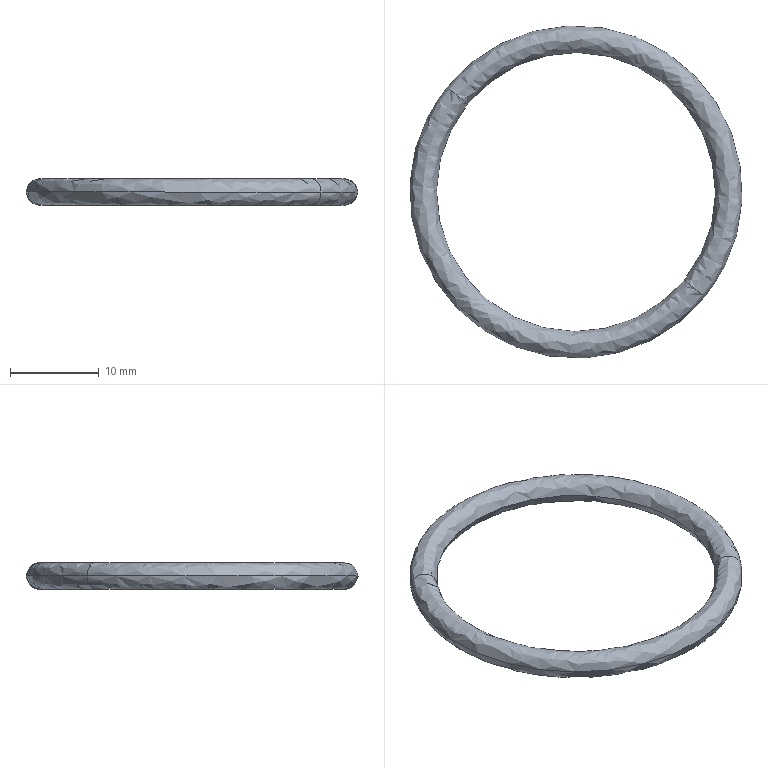Part | SolidWorks | features BaseBody 1 | 1 solid | 4 faces | box 37.4 x 37.4 x 3 mm | volume 763.908 mm3 | spline 4
STEP:
#1=CARTESIAN_POINT('',(521.677,-144.086,275.815));
#2=VERTEX_POINT('',#1);
#3=CARTESIAN_POINT('',(497.316,-124.275,275.815));
#4=VERTEX_POINT('',#3);
#5=CARTESIAN_POINT('',(509.496,-134.18,275.815));
#6=DIRECTION('',(0.000000024,-0.000000004,1.));
#7=DIRECTION('',(-0.7758,0.6309,0.000000021));
#8=AXIS2_PLACEMENT_3D('',#5,#6,#7);
#9=CIRCLE('',#8,15.7);
#10=EDGE_CURVE('',#2,#4,#9,.T.);
#11=ORIENTED_EDGE('',*,*,#10,.F.);
#12=CARTESIAN_POINT('',(524.004,-145.979,275.815));
#13=VERTEX_POINT('',#12);
#14=CARTESIAN_POINT('',(522.841,-145.032,275.815));
#15=DIRECTION('',(0.6309,0.7758,-0.000000012));
#16=DIRECTION('',(0.7758,-0.6309,-0.000000021));
#17=AXIS2_PLACEMENT_3D('',#14,#15,#16);
#18=CIRCLE('',#17,1.5);
#19=EDGE_CURVE('',#2,#13,#18,.T.);
#20=ORIENTED_EDGE('',*,*,#19,.T.);
#21=CARTESIAN_POINT('',(494.988,-122.382,275.815));
#22=VERTEX_POINT('',#21);
#23=CARTESIAN_POINT('',(509.496,-134.18,275.815));
#24=DIRECTION('',(0.000000024,-0.000000004,1.));
#25=DIRECTION('',(-0.7758,0.6309,0.000000021));
#26=AXIS2_PLACEMENT_3D('',#23,#24,#25);
#27=CIRCLE('',#26,18.7);
#28=EDGE_CURVE('',#13,#22,#27,.T.);
#29=ORIENTED_EDGE('',*,*,#28,.T.);
#30=CARTESIAN_POINT('',(496.152,-123.329,275.815));
#31=DIRECTION('',(-0.6309,-0.7758,0.000000012));
#32=DIRECTION('',(-0.7758,0.6309,0.000000021));
#33=AXIS2_PLACEMENT_3D('',#30,#31,#32);
#34=CIRCLE('',#33,1.5);
#35=EDGE_CURVE('',#4,#22,#34,.T.);
#36=ORIENTED_EDGE('',*,*,#35,.F.);
#37=EDGE_LOOP('',(#11,#20,#29,#36));
#38=FACE_OUTER_BOUND('',#37,.T.);
#39=CARTESIAN_POINT('',(521.677,-144.086,275.815));
#40=CARTESIAN_POINT('',(541.488,-119.725,275.815));
#41=CARTESIAN_POINT('',(517.127,-99.914,275.815));
#42=CARTESIAN_POINT('',(497.316,-124.275,275.815));
#43=CARTESIAN_POINT('',(521.677,-144.086,278.815));
#44=CARTESIAN_POINT('',(541.488,-119.725,278.815));
#45=CARTESIAN_POINT('',(517.127,-99.914,278.815));
#46=CARTESIAN_POINT('',(497.316,-124.275,278.815));
#47=CARTESIAN_POINT('',(524.004,-145.979,278.815));
#48=CARTESIAN_POINT('',(547.601,-116.962,278.815));
#49=CARTESIAN_POINT('',(518.585,-93.366,278.815));
#50=CARTESIAN_POINT('',(494.988,-122.382,278.815));
#51=CARTESIAN_POINT('',(524.004,-145.979,275.815));
#52=CARTESIAN_POINT('',(547.601,-116.962,275.815));
#53=CARTESIAN_POINT('',(518.585,-93.366,275.815));
#54=CARTESIAN_POINT('',(494.988,-122.382,275.815));
#55=(BOUNDED_SURFACE()B_SPLINE_SURFACE(3,3,((#39,#40,#41,#42),(#43,#44,#45,#46),(#47,#48,#49,#50),(#51,#52,#53,#54)),.UNSPECIFIED.,.F.,.F.,.F.)B_SPLINE_SURFACE_WITH_KNOTS((4,4),(4,4),(0.,1.),(0.,1.),.UNSPECIFIED.)GEOMETRIC_REPRESENTATION_ITEM()RATIONAL_B_SPLINE_SURFACE(((1.,0.3333,0.3333,1.),(0.3333,0.1111,0.1111,0.3333),(0.3333,0.1111,0.1111,0.3333),(1.,0.3333,0.3333,1.)))REPRESENTATION_ITEM('')SURFACE());
#56=ADVANCED_FACE('',(#38),#55,.T.);
#57=ORIENTED_EDGE('',*,*,#28,.F.);
#58=CARTESIAN_POINT('',(522.841,-145.032,275.815));
#59=DIRECTION('',(0.6309,0.7758,-0.000000012));
#60=DIRECTION('',(0.7758,-0.6309,-0.000000021));
#61=AXIS2_PLACEMENT_3D('',#58,#59,#60);
#62=CIRCLE('',#61,1.5);
#63=EDGE_CURVE('',#13,#2,#62,.T.);
#64=ORIENTED_EDGE('',*,*,#63,.T.);
#65=ORIENTED_EDGE('',*,*,#10,.T.);
#66=CARTESIAN_POINT('',(496.152,-123.329,275.815));
#67=DIRECTION('',(-0.6309,-0.7758,0.000000012));
#68=DIRECTION('',(-0.7758,0.6309,0.000000021));
#69=AXIS2_PLACEMENT_3D('',#66,#67,#68);
#70=CIRCLE('',#69,1.5);
#71=EDGE_CURVE('',#22,#4,#70,.T.);
#72=ORIENTED_EDGE('',*,*,#71,.F.);
#73=EDGE_LOOP('',(#57,#64,#65,#72));
#74=FACE_OUTER_BOUND('',#73,.T.);
#75=CARTESIAN_POINT('',(524.004,-145.979,275.815));
#76=CARTESIAN_POINT('',(547.601,-116.962,275.815));
#77=CARTESIAN_POINT('',(518.585,-93.366,275.815));
#78=CARTESIAN_POINT('',(494.988,-122.382,275.815));
#79=CARTESIAN_POINT('',(524.004,-145.979,272.815));
#80=CARTESIAN_POINT('',(547.601,-116.962,272.815));
#81=CARTESIAN_POINT('',(518.585,-93.366,272.815));
#82=CARTESIAN_POINT('',(494.988,-122.382,272.815));
#83=CARTESIAN_POINT('',(521.677,-144.086,272.815));
#84=CARTESIAN_POINT('',(541.488,-119.725,272.815));
#85=CARTESIAN_POINT('',(517.127,-99.914,272.815));
#86=CARTESIAN_POINT('',(497.316,-124.275,272.815));
#87=CARTESIAN_POINT('',(521.677,-144.086,275.815));
#88=CARTESIAN_POINT('',(541.488,-119.725,275.815));
#89=CARTESIAN_POINT('',(517.127,-99.914,275.815));
#90=CARTESIAN_POINT('',(497.316,-124.275,275.815));
#91=(BOUNDED_SURFACE()B_SPLINE_SURFACE(3,3,((#75,#76,#77,#78),(#79,#80,#81,#82),(#83,#84,#85,#86),(#87,#88,#89,#90)),.UNSPECIFIED.,.F.,.F.,.T.)B_SPLINE_SURFACE_WITH_KNOTS((4,4),(4,4),(0.,1.),(0.,1.),.UNSPECIFIED.)GEOMETRIC_REPRESENTATION_ITEM()RATIONAL_B_SPLINE_SURFACE(((1.,0.3333,0.3333,1.),(0.3333,0.1111,0.1111,0.3333),(0.3333,0.1111,0.1111,0.3333),(1.,0.3333,0.3333,1.)))REPRESENTATION_ITEM('')SURFACE());
#92=ADVANCED_FACE('',(#74),#91,.T.);
#93=ORIENTED_EDGE('',*,*,#63,.F.);
#94=CARTESIAN_POINT('',(509.496,-134.18,275.815));
#95=DIRECTION('',(0.000000024,-0.000000004,1.));
#96=DIRECTION('',(-0.7758,0.6309,0.000000021));
#97=AXIS2_PLACEMENT_3D('',#94,#95,#96);
#98=CIRCLE('',#97,18.7);
#99=EDGE_CURVE('',#22,#13,#98,.T.);
#100=ORIENTED_EDGE('',*,*,#99,.F.);
#101=ORIENTED_EDGE('',*,*,#71,.T.);
#102=CARTESIAN_POINT('',(509.496,-134.18,275.815));
#103=DIRECTION('',(0.000000024,-0.000000004,1.));
#104=DIRECTION('',(-0.7758,0.6309,0.000000021));
#105=AXIS2_PLACEMENT_3D('',#102,#103,#104);
#106=CIRCLE('',#105,15.7);
#107=EDGE_CURVE('',#4,#2,#106,.T.);
#108=ORIENTED_EDGE('',*,*,#107,.T.);
#109=EDGE_LOOP('',(#93,#100,#101,#108));
#110=FACE_OUTER_BOUND('',#109,.T.);
#111=CARTESIAN_POINT('',(494.988,-122.382,275.815));
#112=CARTESIAN_POINT('',(471.391,-151.399,275.815));
#113=CARTESIAN_POINT('',(500.408,-174.995,275.815));
#114=CARTESIAN_POINT('',(524.004,-145.979,275.815));
#115=CARTESIAN_POINT('',(494.988,-122.382,272.815));
#116=CARTESIAN_POINT('',(471.391,-151.399,272.815));
#117=CARTESIAN_POINT('',(500.408,-174.995,272.815));
#118=CARTESIAN_POINT('',(524.004,-145.979,272.815));
#119=CARTESIAN_POINT('',(497.316,-124.275,272.815));
#120=CARTESIAN_POINT('',(477.504,-148.636,272.815));
#121=CARTESIAN_POINT('',(501.866,-168.447,272.815));
#122=CARTESIAN_POINT('',(521.677,-144.086,272.815));
#123=CARTESIAN_POINT('',(497.316,-124.275,275.815));
#124=CARTESIAN_POINT('',(477.504,-148.636,275.815));
#125=CARTESIAN_POINT('',(501.866,-168.447,275.815));
#126=CARTESIAN_POINT('',(521.677,-144.086,275.815));
#127=(BOUNDED_SURFACE()B_SPLINE_SURFACE(3,3,((#111,#112,#113,#114),(#115,#116,#117,#118),(#119,#120,#121,#122),(#123,#124,#125,#126)),.UNSPECIFIED.,.F.,.F.,.F.)B_SPLINE_SURFACE_WITH_KNOTS((4,4),(4,4),(0.,1.),(0.,1.),.UNSPECIFIED.)GEOMETRIC_REPRESENTATION_ITEM()RATIONAL_B_SPLINE_SURFACE(((1.,0.3333,0.3333,1.),(0.3333,0.1111,0.1111,0.3333),(0.3333,0.1111,0.1111,0.3333),(1.,0.3333,0.3333,1.)))REPRESENTATION_ITEM('')SURFACE());
#128=ADVANCED_FACE('',(#110),#127,.T.);
#129=ORIENTED_EDGE('',*,*,#19,.F.);
#130=ORIENTED_EDGE('',*,*,#107,.F.);
#131=ORIENTED_EDGE('',*,*,#35,.T.);
#132=ORIENTED_EDGE('',*,*,#99,.T.);
#133=EDGE_LOOP('',(#129,#130,#131,#132));
#134=FACE_OUTER_BOUND('',#133,.T.);
#135=CARTESIAN_POINT('',(497.316,-124.275,275.815));
#136=CARTESIAN_POINT('',(477.504,-148.636,275.815));
#137=CARTESIAN_POINT('',(501.866,-168.447,275.815));
#138=CARTESIAN_POINT('',(521.677,-144.086,275.815));
#139=CARTESIAN_POINT('',(497.316,-124.275,278.815));
#140=CARTESIAN_POINT('',(477.504,-148.636,278.815));
#141=CARTESIAN_POINT('',(501.866,-168.447,278.815));
#142=CARTESIAN_POINT('',(521.677,-144.086,278.815));
#143=CARTESIAN_POINT('',(494.988,-122.382,278.815));
#144=CARTESIAN_POINT('',(471.391,-151.399,278.815));
#145=CARTESIAN_POINT('',(500.408,-174.995,278.815));
#146=CARTESIAN_POINT('',(524.004,-145.979,278.815));
#147=CARTESIAN_POINT('',(494.988,-122.382,275.815));
#148=CARTESIAN_POINT('',(471.391,-151.399,275.815));
#149=CARTESIAN_POINT('',(500.408,-174.995,275.815));
#150=CARTESIAN_POINT('',(524.004,-145.979,275.815));
#151=(BOUNDED_SURFACE()B_SPLINE_SURFACE(3,3,((#135,#136,#137,#138),(#139,#140,#141,#142),(#143,#144,#145,#146),(#147,#148,#149,#150)),.UNSPECIFIED.,.F.,.F.,.F.)B_SPLINE_SURFACE_WITH_KNOTS((4,4),(4,4),(0.,1.),(0.,1.),.UNSPECIFIED.)GEOMETRIC_REPRESENTATION_ITEM()RATIONAL_B_SPLINE_SURFACE(((1.,0.3333,0.3333,1.),(0.3333,0.1111,0.1111,0.3333),(0.3333,0.1111,0.1111,0.3333),(1.,0.3333,0.3333,1.)))REPRESENTATION_ITEM('')SURFACE());
#152=ADVANCED_FACE('',(#134),#151,.T.);
#153=CLOSED_SHELL('',(#56,#92,#128,#152));
#154=MANIFOLD_SOLID_BREP('',#153);
#155=CARTESIAN_POINT('',(0.,0.,0.));
#156=DIRECTION('',(0.,0.,1.));
#157=DIRECTION('',(1.,0.,0.));
#158=AXIS2_PLACEMENT_3D('',#155,#156,#157);
#159=(LENGTH_UNIT()NAMED_UNIT(*)SI_UNIT(.MILLI.,.METRE.));
#160=UNCERTAINTY_MEASURE_WITH_UNIT(LENGTH_MEASURE(0.00001),#159,'','');
#161=(NAMED_UNIT(*)PLANE_ANGLE_UNIT()SI_UNIT($,.RADIAN.));
#162=(NAMED_UNIT(*)SI_UNIT($,.STERADIAN.)SOLID_ANGLE_UNIT());
#163=(GEOMETRIC_REPRESENTATION_CONTEXT(3)GLOBAL_UNCERTAINTY_ASSIGNED_CONTEXT((#160))GLOBAL_UNIT_ASSIGNED_CONTEXT((#159,#161,#162))REPRESENTATION_CONTEXT('',''));
#164=ADVANCED_BREP_SHAPE_REPRESENTATION('',(#154,#158),#163);